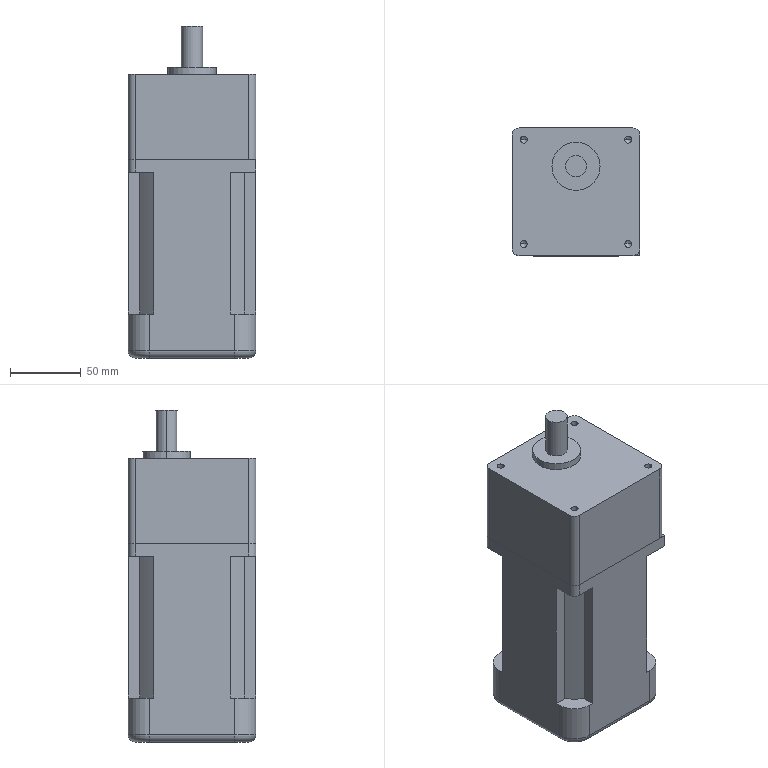Part | NX | features BREP 2 | 2 solids | 73 faces | box 90 x 90 x 234 mm | volume 1510104 mm3 | cylinder 31 | plane 30 | cone 8 | torus 4 | commonest cylinder face diameters 10 x11 5 x8 30 x4 320 x4 15 x2 34 x2